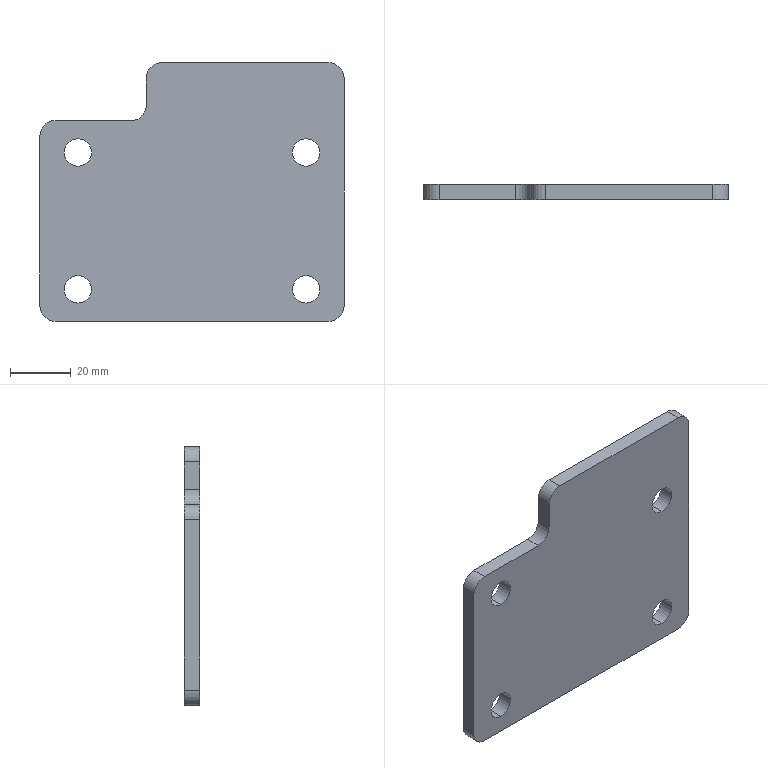Part | SolidWorks | features Fillet 2, Extrusion 1, HoleWzd 1, ICE 1 | 1 solid | 22 faces | box 100 x 5 x 85 mm | volume 37795 mm3 | cylinder 14 | plane 8 | commonest cylinder face diameters 9 x8 10 x6
STEP:
#1=CARTESIAN_POINT('',(-37.5,0.,-36.5));
#2=VERTEX_POINT('',#1);
#3=CARTESIAN_POINT('',(-37.5,0.,-27.5));
#4=VERTEX_POINT('',#3);
#5=CARTESIAN_POINT('',(-37.5,0.,-32.));
#6=DIRECTION('',(0.,1.,0.));
#7=DIRECTION('',(0.,0.,1.));
#8=AXIS2_PLACEMENT_3D('',#5,#6,#7);
#9=CIRCLE('',#8,4.5);
#10=EDGE_CURVE('',#2,#4,#9,.T.);
#11=ORIENTED_EDGE('',*,*,#10,.F.);
#12=CARTESIAN_POINT('',(-37.5,5.,-36.5));
#13=VERTEX_POINT('',#12);
#14=CARTESIAN_POINT('',(-37.5,5.,-36.5));
#15=DIRECTION('',(0.,1.,0.));
#16=VECTOR('',#15,1000.);
#17=LINE('',#14,#16);
#18=EDGE_CURVE('',#2,#13,#17,.T.);
#19=ORIENTED_EDGE('',*,*,#18,.T.);
#20=CARTESIAN_POINT('',(-37.5,5.,-27.5));
#21=VERTEX_POINT('',#20);
#22=CARTESIAN_POINT('',(-37.5,5.,-32.));
#23=DIRECTION('',(0.,1.,0.));
#24=DIRECTION('',(0.,0.,1.));
#25=AXIS2_PLACEMENT_3D('',#22,#23,#24);
#26=CIRCLE('',#25,4.5);
#27=EDGE_CURVE('',#13,#21,#26,.T.);
#28=ORIENTED_EDGE('',*,*,#27,.T.);
#29=CARTESIAN_POINT('',(-37.5,5.,-27.5));
#30=DIRECTION('',(0.,1.,0.));
#31=VECTOR('',#30,1000.);
#32=LINE('',#29,#31);
#33=EDGE_CURVE('',#4,#21,#32,.T.);
#34=ORIENTED_EDGE('',*,*,#33,.F.);
#35=EDGE_LOOP('',(#11,#19,#28,#34));
#36=FACE_OUTER_BOUND('',#35,.T.);
#37=CARTESIAN_POINT('',(-37.5,5.,-32.));
#38=DIRECTION('',(0.,1.,0.));
#39=DIRECTION('',(0.,0.,1.));
#40=AXIS2_PLACEMENT_3D('',#37,#38,#39);
#41=CYLINDRICAL_SURFACE('',#40,4.5);
#42=ADVANCED_FACE('',(#36),#41,.F.);
#43=CARTESIAN_POINT('',(37.5,0.,-36.5));
#44=VERTEX_POINT('',#43);
#45=CARTESIAN_POINT('',(37.5,0.,-27.5));
#46=VERTEX_POINT('',#45);
#47=CARTESIAN_POINT('',(37.5,0.,-32.));
#48=DIRECTION('',(0.,1.,0.));
#49=DIRECTION('',(0.,0.,1.));
#50=AXIS2_PLACEMENT_3D('',#47,#48,#49);
#51=CIRCLE('',#50,4.5);
#52=EDGE_CURVE('',#44,#46,#51,.T.);
#53=ORIENTED_EDGE('',*,*,#52,.F.);
#54=CARTESIAN_POINT('',(37.5,5.,-36.5));
#55=VERTEX_POINT('',#54);
#56=CARTESIAN_POINT('',(37.5,5.,-36.5));
#57=DIRECTION('',(0.,1.,0.));
#58=VECTOR('',#57,1000.);
#59=LINE('',#56,#58);
#60=EDGE_CURVE('',#44,#55,#59,.T.);
#61=ORIENTED_EDGE('',*,*,#60,.T.);
#62=CARTESIAN_POINT('',(37.5,5.,-27.5));
#63=VERTEX_POINT('',#62);
#64=CARTESIAN_POINT('',(37.5,5.,-32.));
#65=DIRECTION('',(0.,1.,0.));
#66=DIRECTION('',(0.,0.,1.));
#67=AXIS2_PLACEMENT_3D('',#64,#65,#66);
#68=CIRCLE('',#67,4.5);
#69=EDGE_CURVE('',#55,#63,#68,.T.);
#70=ORIENTED_EDGE('',*,*,#69,.T.);
#71=CARTESIAN_POINT('',(37.5,5.,-27.5));
#72=DIRECTION('',(0.,1.,0.));
#73=VECTOR('',#72,1000.);
#74=LINE('',#71,#73);
#75=EDGE_CURVE('',#46,#63,#74,.T.);
#76=ORIENTED_EDGE('',*,*,#75,.F.);
#77=EDGE_LOOP('',(#53,#61,#70,#76));
#78=FACE_OUTER_BOUND('',#77,.T.);
#79=CARTESIAN_POINT('',(37.5,5.,-32.));
#80=DIRECTION('',(0.,1.,0.));
#81=DIRECTION('',(0.,0.,1.));
#82=AXIS2_PLACEMENT_3D('',#79,#80,#81);
#83=CYLINDRICAL_SURFACE('',#82,4.5);
#84=ADVANCED_FACE('',(#78),#83,.F.);
#85=CARTESIAN_POINT('',(37.5,0.,8.5));
#86=VERTEX_POINT('',#85);
#87=CARTESIAN_POINT('',(37.5,0.,17.5));
#88=VERTEX_POINT('',#87);
#89=CARTESIAN_POINT('',(37.5,0.,13.));
#90=DIRECTION('',(0.,1.,0.));
#91=DIRECTION('',(0.,0.,1.));
#92=AXIS2_PLACEMENT_3D('',#89,#90,#91);
#93=CIRCLE('',#92,4.5);
#94=EDGE_CURVE('',#86,#88,#93,.T.);
#95=ORIENTED_EDGE('',*,*,#94,.F.);
#96=CARTESIAN_POINT('',(37.5,5.,8.5));
#97=VERTEX_POINT('',#96);
#98=CARTESIAN_POINT('',(37.5,5.,8.5));
#99=DIRECTION('',(0.,1.,0.));
#100=VECTOR('',#99,1000.);
#101=LINE('',#98,#100);
#102=EDGE_CURVE('',#86,#97,#101,.T.);
#103=ORIENTED_EDGE('',*,*,#102,.T.);
#104=CARTESIAN_POINT('',(37.5,5.,17.5));
#105=VERTEX_POINT('',#104);
#106=CARTESIAN_POINT('',(37.5,5.,13.));
#107=DIRECTION('',(0.,1.,0.));
#108=DIRECTION('',(0.,0.,1.));
#109=AXIS2_PLACEMENT_3D('',#106,#107,#108);
#110=CIRCLE('',#109,4.5);
#111=EDGE_CURVE('',#97,#105,#110,.T.);
#112=ORIENTED_EDGE('',*,*,#111,.T.);
#113=CARTESIAN_POINT('',(37.5,5.,17.5));
#114=DIRECTION('',(0.,1.,0.));
#115=VECTOR('',#114,1000.);
#116=LINE('',#113,#115);
#117=EDGE_CURVE('',#88,#105,#116,.T.);
#118=ORIENTED_EDGE('',*,*,#117,.F.);
#119=EDGE_LOOP('',(#95,#103,#112,#118));
#120=FACE_OUTER_BOUND('',#119,.T.);
#121=CARTESIAN_POINT('',(37.5,5.,13.));
#122=DIRECTION('',(0.,1.,0.));
#123=DIRECTION('',(0.,0.,1.));
#124=AXIS2_PLACEMENT_3D('',#121,#122,#123);
#125=CYLINDRICAL_SURFACE('',#124,4.5);
#126=ADVANCED_FACE('',(#120),#125,.F.);
#127=CARTESIAN_POINT('',(-37.5,0.,8.5));
#128=VERTEX_POINT('',#127);
#129=CARTESIAN_POINT('',(-37.5,0.,17.5));
#130=VERTEX_POINT('',#129);
#131=CARTESIAN_POINT('',(-37.5,0.,13.));
#132=DIRECTION('',(0.,1.,0.));
#133=DIRECTION('',(0.,0.,1.));
#134=AXIS2_PLACEMENT_3D('',#131,#132,#133);
#135=CIRCLE('',#134,4.5);
#136=EDGE_CURVE('',#128,#130,#135,.T.);
#137=ORIENTED_EDGE('',*,*,#136,.F.);
#138=CARTESIAN_POINT('',(-37.5,5.,8.5));
#139=VERTEX_POINT('',#138);
#140=CARTESIAN_POINT('',(-37.5,5.,8.5));
#141=DIRECTION('',(0.,1.,0.));
#142=VECTOR('',#141,1000.);
#143=LINE('',#140,#142);
#144=EDGE_CURVE('',#128,#139,#143,.T.);
#145=ORIENTED_EDGE('',*,*,#144,.T.);
#146=CARTESIAN_POINT('',(-37.5,5.,17.5));
#147=VERTEX_POINT('',#146);
#148=CARTESIAN_POINT('',(-37.5,5.,13.));
#149=DIRECTION('',(0.,1.,0.));
#150=DIRECTION('',(0.,0.,1.));
#151=AXIS2_PLACEMENT_3D('',#148,#149,#150);
#152=CIRCLE('',#151,4.5);
#153=EDGE_CURVE('',#139,#147,#152,.T.);
#154=ORIENTED_EDGE('',*,*,#153,.T.);
#155=CARTESIAN_POINT('',(-37.5,5.,17.5));
#156=DIRECTION('',(0.,1.,0.));
#157=VECTOR('',#156,1000.);
#158=LINE('',#155,#157);
#159=EDGE_CURVE('',#130,#147,#158,.T.);
#160=ORIENTED_EDGE('',*,*,#159,.F.);
#161=EDGE_LOOP('',(#137,#145,#154,#160));
#162=FACE_OUTER_BOUND('',#161,.T.);
#163=CARTESIAN_POINT('',(-37.5,5.,13.));
#164=DIRECTION('',(0.,1.,0.));
#165=DIRECTION('',(0.,0.,1.));
#166=AXIS2_PLACEMENT_3D('',#163,#164,#165);
#167=CYLINDRICAL_SURFACE('',#166,4.5);
#168=ADVANCED_FACE('',(#162),#167,.F.);
#169=CARTESIAN_POINT('',(50.,5.,37.5));
#170=VERTEX_POINT('',#169);
#171=CARTESIAN_POINT('',(50.,5.,-37.5));
#172=VERTEX_POINT('',#171);
#173=CARTESIAN_POINT('',(50.,5.,-42.5));
#174=DIRECTION('',(0.,0.,-1.));
#175=VECTOR('',#174,1000.);
#176=LINE('',#173,#175);
#177=EDGE_CURVE('',#170,#172,#176,.T.);
#178=ORIENTED_EDGE('',*,*,#177,.F.);
#179=CARTESIAN_POINT('',(50.,0.,37.5));
#180=VERTEX_POINT('',#179);
#181=CARTESIAN_POINT('',(50.,5.,37.5));
#182=DIRECTION('',(0.,-1.,0.));
#183=VECTOR('',#182,1000.);
#184=LINE('',#181,#183);
#185=EDGE_CURVE('',#170,#180,#184,.T.);
#186=ORIENTED_EDGE('',*,*,#185,.T.);
#187=CARTESIAN_POINT('',(50.,0.,-37.5));
#188=VERTEX_POINT('',#187);
#189=CARTESIAN_POINT('',(50.,0.,-42.5));
#190=DIRECTION('',(0.,0.,-1.));
#191=VECTOR('',#190,1000.);
#192=LINE('',#189,#191);
#193=EDGE_CURVE('',#180,#188,#192,.T.);
#194=ORIENTED_EDGE('',*,*,#193,.T.);
#195=CARTESIAN_POINT('',(50.,5.,-37.5));
#196=DIRECTION('',(0.,1.,0.));
#197=VECTOR('',#196,1000.);
#198=LINE('',#195,#197);
#199=EDGE_CURVE('',#188,#172,#198,.T.);
#200=ORIENTED_EDGE('',*,*,#199,.T.);
#201=EDGE_LOOP('',(#178,#186,#194,#200));
#202=FACE_OUTER_BOUND('',#201,.T.);
#203=CARTESIAN_POINT('',(50.,5.,-42.5));
#204=DIRECTION('',(-1.,0.,0.));
#205=DIRECTION('',(0.,0.,1.));
#206=AXIS2_PLACEMENT_3D('',#203,#204,#205);
#207=PLANE('',#206);
#208=ADVANCED_FACE('',(#202),#207,.F.);
#209=CARTESIAN_POINT('',(45.,5.,-42.5));
#210=VERTEX_POINT('',#209);
#211=CARTESIAN_POINT('',(-45.,5.,-42.5));
#212=VERTEX_POINT('',#211);
#213=CARTESIAN_POINT('',(-50.,5.,-42.5));
#214=DIRECTION('',(-1.,0.,0.));
#215=VECTOR('',#214,1000.);
#216=LINE('',#213,#215);
#217=EDGE_CURVE('',#210,#212,#216,.T.);
#218=ORIENTED_EDGE('',*,*,#217,.F.);
#219=CARTESIAN_POINT('',(45.,0.,-42.5));
#220=VERTEX_POINT('',#219);
#221=CARTESIAN_POINT('',(45.,5.,-42.5));
#222=DIRECTION('',(0.,-1.,0.));
#223=VECTOR('',#222,1000.);
#224=LINE('',#221,#223);
#225=EDGE_CURVE('',#210,#220,#224,.T.);
#226=ORIENTED_EDGE('',*,*,#225,.T.);
#227=CARTESIAN_POINT('',(-45.,0.,-42.5));
#228=VERTEX_POINT('',#227);
#229=CARTESIAN_POINT('',(-50.,0.,-42.5));
#230=DIRECTION('',(-1.,0.,0.));
#231=VECTOR('',#230,1000.);
#232=LINE('',#229,#231);
#233=EDGE_CURVE('',#220,#228,#232,.T.);
#234=ORIENTED_EDGE('',*,*,#233,.T.);
#235=CARTESIAN_POINT('',(-45.,5.,-42.5));
#236=DIRECTION('',(0.,1.,0.));
#237=VECTOR('',#236,1000.);
#238=LINE('',#235,#237);
#239=EDGE_CURVE('',#228,#212,#238,.T.);
#240=ORIENTED_EDGE('',*,*,#239,.T.);
#241=EDGE_LOOP('',(#218,#226,#234,#240));
#242=FACE_OUTER_BOUND('',#241,.T.);
#243=CARTESIAN_POINT('',(-50.,5.,-42.5));
#244=DIRECTION('',(0.,0.,1.));
#245=DIRECTION('',(1.,0.,0.));
#246=AXIS2_PLACEMENT_3D('',#243,#244,#245);
#247=PLANE('',#246);
#248=ADVANCED_FACE('',(#242),#247,.F.);
#249=CARTESIAN_POINT('',(-50.,0.,-37.5));
#250=VERTEX_POINT('',#249);
#251=CARTESIAN_POINT('',(-50.,0.,18.5));
#252=VERTEX_POINT('',#251);
#253=CARTESIAN_POINT('',(-50.,0.,-42.5));
#254=DIRECTION('',(0.,0.,1.));
#255=VECTOR('',#254,1000.);
#256=LINE('',#253,#255);
#257=EDGE_CURVE('',#250,#252,#256,.T.);
#258=ORIENTED_EDGE('',*,*,#257,.T.);
#259=CARTESIAN_POINT('',(-50.,5.,18.5));
#260=VERTEX_POINT('',#259);
#261=CARTESIAN_POINT('',(-50.,5.,18.5));
#262=DIRECTION('',(0.,1.,0.));
#263=VECTOR('',#262,1000.);
#264=LINE('',#261,#263);
#265=EDGE_CURVE('',#252,#260,#264,.T.);
#266=ORIENTED_EDGE('',*,*,#265,.T.);
#267=CARTESIAN_POINT('',(-50.,5.,-37.5));
#268=VERTEX_POINT('',#267);
#269=CARTESIAN_POINT('',(-50.,5.,-42.5));
#270=DIRECTION('',(0.,0.,1.));
#271=VECTOR('',#270,1000.);
#272=LINE('',#269,#271);
#273=EDGE_CURVE('',#268,#260,#272,.T.);
#274=ORIENTED_EDGE('',*,*,#273,.F.);
#275=CARTESIAN_POINT('',(-50.,5.,-37.5));
#276=DIRECTION('',(0.,-1.,0.));
#277=VECTOR('',#276,1000.);
#278=LINE('',#275,#277);
#279=EDGE_CURVE('',#268,#250,#278,.T.);
#280=ORIENTED_EDGE('',*,*,#279,.T.);
#281=EDGE_LOOP('',(#258,#266,#274,#280));
#282=FACE_OUTER_BOUND('',#281,.T.);
#283=CARTESIAN_POINT('',(-50.,5.,-42.5));
#284=DIRECTION('',(1.,0.,0.));
#285=DIRECTION('',(0.,0.,-1.));
#286=AXIS2_PLACEMENT_3D('',#283,#284,#285);
#287=PLANE('',#286);
#288=ADVANCED_FACE('',(#282),#287,.F.);
#289=CARTESIAN_POINT('',(-10.,5.,42.5));
#290=VERTEX_POINT('',#289);
#291=CARTESIAN_POINT('',(45.,5.,42.5));
#292=VERTEX_POINT('',#291);
#293=CARTESIAN_POINT('',(-50.,5.,42.5));
#294=DIRECTION('',(1.,0.,0.));
#295=VECTOR('',#294,1000.);
#296=LINE('',#293,#295);
#297=EDGE_CURVE('',#290,#292,#296,.T.);
#298=ORIENTED_EDGE('',*,*,#297,.F.);
#299=CARTESIAN_POINT('',(-10.,0.,42.5));
#300=VERTEX_POINT('',#299);
#301=CARTESIAN_POINT('',(-10.,5.,42.5));
#302=DIRECTION('',(0.,-1.,0.));
#303=VECTOR('',#302,1000.);
#304=LINE('',#301,#303);
#305=EDGE_CURVE('',#290,#300,#304,.T.);
#306=ORIENTED_EDGE('',*,*,#305,.T.);
#307=CARTESIAN_POINT('',(45.,0.,42.5));
#308=VERTEX_POINT('',#307);
#309=CARTESIAN_POINT('',(-50.,0.,42.5));
#310=DIRECTION('',(1.,0.,0.));
#311=VECTOR('',#310,1000.);
#312=LINE('',#309,#311);
#313=EDGE_CURVE('',#300,#308,#312,.T.);
#314=ORIENTED_EDGE('',*,*,#313,.T.);
#315=CARTESIAN_POINT('',(45.,5.,42.5));
#316=DIRECTION('',(0.,1.,0.));
#317=VECTOR('',#316,1000.);
#318=LINE('',#315,#317);
#319=EDGE_CURVE('',#308,#292,#318,.T.);
#320=ORIENTED_EDGE('',*,*,#319,.T.);
#321=EDGE_LOOP('',(#298,#306,#314,#320));
#322=FACE_OUTER_BOUND('',#321,.T.);
#323=CARTESIAN_POINT('',(-50.,5.,42.5));
#324=DIRECTION('',(0.,0.,-1.));
#325=DIRECTION('',(-1.,0.,0.));
#326=AXIS2_PLACEMENT_3D('',#323,#324,#325);
#327=PLANE('',#326);
#328=ADVANCED_FACE('',(#322),#327,.F.);
#329=CARTESIAN_POINT('',(-15.,5.,37.5));
#330=VERTEX_POINT('',#329);
#331=CARTESIAN_POINT('',(-15.,5.,28.5));
#332=VERTEX_POINT('',#331);
#333=CARTESIAN_POINT('',(-15.,5.,42.5));
#334=DIRECTION('',(0.,0.,-1.));
#335=VECTOR('',#334,1000.);
#336=LINE('',#333,#335);
#337=EDGE_CURVE('',#330,#332,#336,.T.);
#338=ORIENTED_EDGE('',*,*,#337,.F.);
#339=CARTESIAN_POINT('',(-10.,5.,37.5));
#340=DIRECTION('',(0.,1.,0.));
#341=DIRECTION('',(0.,0.,1.));
#342=AXIS2_PLACEMENT_3D('',#339,#340,#341);
#343=CIRCLE('',#342,5.);
#344=EDGE_CURVE('',#330,#290,#343,.T.);
#345=ORIENTED_EDGE('',*,*,#344,.T.);
#346=ORIENTED_EDGE('',*,*,#297,.T.);
#347=CARTESIAN_POINT('',(45.,5.,37.5));
#348=DIRECTION('',(0.,1.,0.));
#349=DIRECTION('',(0.,0.,1.));
#350=AXIS2_PLACEMENT_3D('',#347,#348,#349);
#351=CIRCLE('',#350,5.);
#352=EDGE_CURVE('',#292,#170,#351,.T.);
#353=ORIENTED_EDGE('',*,*,#352,.T.);
#354=ORIENTED_EDGE('',*,*,#177,.T.);
#355=CARTESIAN_POINT('',(45.,5.,-37.5));
#356=DIRECTION('',(0.,1.,0.));
#357=DIRECTION('',(0.,0.,1.));
#358=AXIS2_PLACEMENT_3D('',#355,#356,#357);
#359=CIRCLE('',#358,5.);
#360=EDGE_CURVE('',#172,#210,#359,.T.);
#361=ORIENTED_EDGE('',*,*,#360,.T.);
#362=ORIENTED_EDGE('',*,*,#217,.T.);
#363=CARTESIAN_POINT('',(-45.,5.,-37.5));
#364=DIRECTION('',(0.,1.,0.));
#365=DIRECTION('',(0.,0.,1.));
#366=AXIS2_PLACEMENT_3D('',#363,#364,#365);
#367=CIRCLE('',#366,5.);
#368=EDGE_CURVE('',#212,#268,#367,.T.);
#369=ORIENTED_EDGE('',*,*,#368,.T.);
#370=ORIENTED_EDGE('',*,*,#273,.T.);
#371=CARTESIAN_POINT('',(-45.,5.,23.5));
#372=VERTEX_POINT('',#371);
#373=CARTESIAN_POINT('',(-45.,5.,18.5));
#374=DIRECTION('',(0.,1.,0.));
#375=DIRECTION('',(0.,0.,1.));
#376=AXIS2_PLACEMENT_3D('',#373,#374,#375);
#377=CIRCLE('',#376,5.);
#378=EDGE_CURVE('',#260,#372,#377,.T.);
#379=ORIENTED_EDGE('',*,*,#378,.T.);
#380=CARTESIAN_POINT('',(-20.,5.,23.5));
#381=VERTEX_POINT('',#380);
#382=CARTESIAN_POINT('',(-50.,5.,23.5));
#383=DIRECTION('',(-1.,0.,0.));
#384=VECTOR('',#383,1000.);
#385=LINE('',#382,#384);
#386=EDGE_CURVE('',#381,#372,#385,.T.);
#387=ORIENTED_EDGE('',*,*,#386,.F.);
#388=CARTESIAN_POINT('',(-20.,5.,28.5));
#389=DIRECTION('',(0.,-1.,0.));
#390=DIRECTION('',(0.,0.,1.));
#391=AXIS2_PLACEMENT_3D('',#388,#389,#390);
#392=CIRCLE('',#391,5.);
#393=EDGE_CURVE('',#381,#332,#392,.T.);
#394=ORIENTED_EDGE('',*,*,#393,.T.);
#395=EDGE_LOOP('',(#338,#345,#346,#353,#354,#361,#362,#369,#370,#379,#387,#394));
#396=FACE_OUTER_BOUND('',#395,.T.);
#397=CARTESIAN_POINT('',(-37.5,5.,-32.));
#398=DIRECTION('',(0.,1.,0.));
#399=DIRECTION('',(0.,0.,1.));
#400=AXIS2_PLACEMENT_3D('',#397,#398,#399);
#401=CIRCLE('',#400,4.5);
#402=EDGE_CURVE('',#21,#13,#401,.T.);
#403=ORIENTED_EDGE('',*,*,#402,.F.);
#404=ORIENTED_EDGE('',*,*,#27,.F.);
#405=EDGE_LOOP('',(#403,#404));
#406=FACE_BOUND('',#405,.T.);
#407=CARTESIAN_POINT('',(37.5,5.,-32.));
#408=DIRECTION('',(0.,1.,0.));
#409=DIRECTION('',(0.,0.,1.));
#410=AXIS2_PLACEMENT_3D('',#407,#408,#409);
#411=CIRCLE('',#410,4.5);
#412=EDGE_CURVE('',#63,#55,#411,.T.);
#413=ORIENTED_EDGE('',*,*,#412,.F.);
#414=ORIENTED_EDGE('',*,*,#69,.F.);
#415=EDGE_LOOP('',(#413,#414));
#416=FACE_BOUND('',#415,.T.);
#417=CARTESIAN_POINT('',(37.5,5.,13.));
#418=DIRECTION('',(0.,1.,0.));
#419=DIRECTION('',(0.,0.,1.));
#420=AXIS2_PLACEMENT_3D('',#417,#418,#419);
#421=CIRCLE('',#420,4.5);
#422=EDGE_CURVE('',#105,#97,#421,.T.);
#423=ORIENTED_EDGE('',*,*,#422,.F.);
#424=ORIENTED_EDGE('',*,*,#111,.F.);
#425=EDGE_LOOP('',(#423,#424));
#426=FACE_BOUND('',#425,.T.);
#427=CARTESIAN_POINT('',(-37.5,5.,13.));
#428=DIRECTION('',(0.,1.,0.));
#429=DIRECTION('',(0.,0.,1.));
#430=AXIS2_PLACEMENT_3D('',#427,#428,#429);
#431=CIRCLE('',#430,4.5);
#432=EDGE_CURVE('',#147,#139,#431,.T.);
#433=ORIENTED_EDGE('',*,*,#432,.F.);
#434=ORIENTED_EDGE('',*,*,#153,.F.);
#435=EDGE_LOOP('',(#433,#434));
#436=FACE_BOUND('',#435,.T.);
#437=CARTESIAN_POINT('',(0.,5.,0.));
#438=DIRECTION('',(0.,1.,0.));
#439=DIRECTION('',(0.,0.,1.));
#440=AXIS2_PLACEMENT_3D('',#437,#438,#439);
#441=PLANE('',#440);
#442=ADVANCED_FACE('',(#396,#406,#416,#426,#436),#441,.T.);
#443=CARTESIAN_POINT('',(-37.5,0.,-32.));
#444=DIRECTION('',(0.,1.,0.));
#445=DIRECTION('',(0.,0.,1.));
#446=AXIS2_PLACEMENT_3D('',#443,#444,#445);
#447=CIRCLE('',#446,4.5);
#448=EDGE_CURVE('',#4,#2,#447,.T.);
#449=ORIENTED_EDGE('',*,*,#448,.T.);
#450=ORIENTED_EDGE('',*,*,#10,.T.);
#451=EDGE_LOOP('',(#449,#450));
#452=FACE_BOUND('',#451,.T.);
#453=CARTESIAN_POINT('',(37.5,0.,-32.));
#454=DIRECTION('',(0.,1.,0.));
#455=DIRECTION('',(0.,0.,1.));
#456=AXIS2_PLACEMENT_3D('',#453,#454,#455);
#457=CIRCLE('',#456,4.5);
#458=EDGE_CURVE('',#46,#44,#457,.T.);
#459=ORIENTED_EDGE('',*,*,#458,.T.);
#460=ORIENTED_EDGE('',*,*,#52,.T.);
#461=EDGE_LOOP('',(#459,#460));
#462=FACE_BOUND('',#461,.T.);
#463=CARTESIAN_POINT('',(37.5,0.,13.));
#464=DIRECTION('',(0.,1.,0.));
#465=DIRECTION('',(0.,0.,1.));
#466=AXIS2_PLACEMENT_3D('',#463,#464,#465);
#467=CIRCLE('',#466,4.5);
#468=EDGE_CURVE('',#88,#86,#467,.T.);
#469=ORIENTED_EDGE('',*,*,#468,.T.);
#470=ORIENTED_EDGE('',*,*,#94,.T.);
#471=EDGE_LOOP('',(#469,#470));
#472=FACE_BOUND('',#471,.T.);
#473=CARTESIAN_POINT('',(-37.5,0.,13.));
#474=DIRECTION('',(0.,1.,0.));
#475=DIRECTION('',(0.,0.,1.));
#476=AXIS2_PLACEMENT_3D('',#473,#474,#475);
#477=CIRCLE('',#476,4.5);
#478=EDGE_CURVE('',#130,#128,#477,.T.);
#479=ORIENTED_EDGE('',*,*,#478,.T.);
#480=ORIENTED_EDGE('',*,*,#136,.T.);
#481=EDGE_LOOP('',(#479,#480));
#482=FACE_BOUND('',#481,.T.);
#483=ORIENTED_EDGE('',*,*,#313,.F.);
#484=CARTESIAN_POINT('',(-15.,0.,37.5));
#485=VERTEX_POINT('',#484);
#486=CARTESIAN_POINT('',(-10.,0.,37.5));
#487=DIRECTION('',(0.,-1.,0.));
#488=DIRECTION('',(0.,0.,1.));
#489=AXIS2_PLACEMENT_3D('',#486,#487,#488);
#490=CIRCLE('',#489,5.);
#491=EDGE_CURVE('',#300,#485,#490,.T.);
#492=ORIENTED_EDGE('',*,*,#491,.T.);
#493=CARTESIAN_POINT('',(-15.,0.,28.5));
#494=VERTEX_POINT('',#493);
#495=CARTESIAN_POINT('',(-15.,0.,42.5));
#496=DIRECTION('',(0.,0.,-1.));
#497=VECTOR('',#496,1000.);
#498=LINE('',#495,#497);
#499=EDGE_CURVE('',#485,#494,#498,.T.);
#500=ORIENTED_EDGE('',*,*,#499,.T.);
#501=CARTESIAN_POINT('',(-20.,0.,23.5));
#502=VERTEX_POINT('',#501);
#503=CARTESIAN_POINT('',(-20.,0.,28.5));
#504=DIRECTION('',(0.,1.,0.));
#505=DIRECTION('',(0.,0.,1.));
#506=AXIS2_PLACEMENT_3D('',#503,#504,#505);
#507=CIRCLE('',#506,5.);
#508=EDGE_CURVE('',#494,#502,#507,.T.);
#509=ORIENTED_EDGE('',*,*,#508,.T.);
#510=CARTESIAN_POINT('',(-45.,0.,23.5));
#511=VERTEX_POINT('',#510);
#512=CARTESIAN_POINT('',(-50.,0.,23.5));
#513=DIRECTION('',(-1.,0.,0.));
#514=VECTOR('',#513,1000.);
#515=LINE('',#512,#514);
#516=EDGE_CURVE('',#502,#511,#515,.T.);
#517=ORIENTED_EDGE('',*,*,#516,.T.);
#518=CARTESIAN_POINT('',(-45.,0.,18.5));
#519=DIRECTION('',(0.,-1.,0.));
#520=DIRECTION('',(0.,0.,1.));
#521=AXIS2_PLACEMENT_3D('',#518,#519,#520);
#522=CIRCLE('',#521,5.);
#523=EDGE_CURVE('',#511,#252,#522,.T.);
#524=ORIENTED_EDGE('',*,*,#523,.T.);
#525=ORIENTED_EDGE('',*,*,#257,.F.);
#526=CARTESIAN_POINT('',(-45.,0.,-37.5));
#527=DIRECTION('',(0.,-1.,0.));
#528=DIRECTION('',(0.,0.,1.));
#529=AXIS2_PLACEMENT_3D('',#526,#527,#528);
#530=CIRCLE('',#529,5.);
#531=EDGE_CURVE('',#250,#228,#530,.T.);
#532=ORIENTED_EDGE('',*,*,#531,.T.);
#533=ORIENTED_EDGE('',*,*,#233,.F.);
#534=CARTESIAN_POINT('',(45.,0.,-37.5));
#535=DIRECTION('',(0.,-1.,0.));
#536=DIRECTION('',(0.,0.,1.));
#537=AXIS2_PLACEMENT_3D('',#534,#535,#536);
#538=CIRCLE('',#537,5.);
#539=EDGE_CURVE('',#220,#188,#538,.T.);
#540=ORIENTED_EDGE('',*,*,#539,.T.);
#541=ORIENTED_EDGE('',*,*,#193,.F.);
#542=CARTESIAN_POINT('',(45.,0.,37.5));
#543=DIRECTION('',(0.,-1.,0.));
#544=DIRECTION('',(0.,0.,1.));
#545=AXIS2_PLACEMENT_3D('',#542,#543,#544);
#546=CIRCLE('',#545,5.);
#547=EDGE_CURVE('',#180,#308,#546,.T.);
#548=ORIENTED_EDGE('',*,*,#547,.T.);
#549=EDGE_LOOP('',(#483,#492,#500,#509,#517,#524,#525,#532,#533,#540,#541,#548));
#550=FACE_OUTER_BOUND('',#549,.T.);
#551=CARTESIAN_POINT('',(0.,0.,0.));
#552=DIRECTION('',(0.,1.,0.));
#553=DIRECTION('',(0.,0.,1.));
#554=AXIS2_PLACEMENT_3D('',#551,#552,#553);
#555=PLANE('',#554);
#556=ADVANCED_FACE('',(#452,#462,#472,#482,#550),#555,.F.);
#557=ORIENTED_EDGE('',*,*,#144,.F.);
#558=ORIENTED_EDGE('',*,*,#478,.F.);
#559=ORIENTED_EDGE('',*,*,#159,.T.);
#560=ORIENTED_EDGE('',*,*,#432,.T.);
#561=EDGE_LOOP('',(#557,#558,#559,#560));
#562=FACE_OUTER_BOUND('',#561,.T.);
#563=CARTESIAN_POINT('',(-37.5,5.,13.));
#564=DIRECTION('',(0.,1.,0.));
#565=DIRECTION('',(0.,0.,1.));
#566=AXIS2_PLACEMENT_3D('',#563,#564,#565);
#567=CYLINDRICAL_SURFACE('',#566,4.5);
#568=ADVANCED_FACE('',(#562),#567,.F.);
#569=ORIENTED_EDGE('',*,*,#102,.F.);
#570=ORIENTED_EDGE('',*,*,#468,.F.);
#571=ORIENTED_EDGE('',*,*,#117,.T.);
#572=ORIENTED_EDGE('',*,*,#422,.T.);
#573=EDGE_LOOP('',(#569,#570,#571,#572));
#574=FACE_OUTER_BOUND('',#573,.T.);
#575=CARTESIAN_POINT('',(37.5,5.,13.));
#576=DIRECTION('',(0.,1.,0.));
#577=DIRECTION('',(0.,0.,1.));
#578=AXIS2_PLACEMENT_3D('',#575,#576,#577);
#579=CYLINDRICAL_SURFACE('',#578,4.5);
#580=ADVANCED_FACE('',(#574),#579,.F.);
#581=ORIENTED_EDGE('',*,*,#60,.F.);
#582=ORIENTED_EDGE('',*,*,#458,.F.);
#583=ORIENTED_EDGE('',*,*,#75,.T.);
#584=ORIENTED_EDGE('',*,*,#412,.T.);
#585=EDGE_LOOP('',(#581,#582,#583,#584));
#586=FACE_OUTER_BOUND('',#585,.T.);
#587=CARTESIAN_POINT('',(37.5,5.,-32.));
#588=DIRECTION('',(0.,1.,0.));
#589=DIRECTION('',(0.,0.,1.));
#590=AXIS2_PLACEMENT_3D('',#587,#588,#589);
#591=CYLINDRICAL_SURFACE('',#590,4.5);
#592=ADVANCED_FACE('',(#586),#591,.F.);
#593=ORIENTED_EDGE('',*,*,#18,.F.);
#594=ORIENTED_EDGE('',*,*,#448,.F.);
#595=ORIENTED_EDGE('',*,*,#33,.T.);
#596=ORIENTED_EDGE('',*,*,#402,.T.);
#597=EDGE_LOOP('',(#593,#594,#595,#596));
#598=FACE_OUTER_BOUND('',#597,.T.);
#599=CARTESIAN_POINT('',(-37.5,5.,-32.));
#600=DIRECTION('',(0.,1.,0.));
#601=DIRECTION('',(0.,0.,1.));
#602=AXIS2_PLACEMENT_3D('',#599,#600,#601);
#603=CYLINDRICAL_SURFACE('',#602,4.5);
#604=ADVANCED_FACE('',(#598),#603,.F.);
#605=ORIENTED_EDGE('',*,*,#352,.F.);
#606=ORIENTED_EDGE('',*,*,#319,.F.);
#607=ORIENTED_EDGE('',*,*,#547,.F.);
#608=ORIENTED_EDGE('',*,*,#185,.F.);
#609=EDGE_LOOP('',(#605,#606,#607,#608));
#610=FACE_OUTER_BOUND('',#609,.T.);
#611=CARTESIAN_POINT('',(45.,5.,37.5));
#612=DIRECTION('',(0.,-1.,0.));
#613=DIRECTION('',(0.,0.,-1.));
#614=AXIS2_PLACEMENT_3D('',#611,#612,#613);
#615=CYLINDRICAL_SURFACE('',#614,5.);
#616=ADVANCED_FACE('',(#610),#615,.T.);
#617=ORIENTED_EDGE('',*,*,#360,.F.);
#618=ORIENTED_EDGE('',*,*,#199,.F.);
#619=ORIENTED_EDGE('',*,*,#539,.F.);
#620=ORIENTED_EDGE('',*,*,#225,.F.);
#621=EDGE_LOOP('',(#617,#618,#619,#620));
#622=FACE_OUTER_BOUND('',#621,.T.);
#623=CARTESIAN_POINT('',(45.,5.,-37.5));
#624=DIRECTION('',(0.,-1.,0.));
#625=DIRECTION('',(0.,0.,-1.));
#626=AXIS2_PLACEMENT_3D('',#623,#624,#625);
#627=CYLINDRICAL_SURFACE('',#626,5.);
#628=ADVANCED_FACE('',(#622),#627,.T.);
#629=ORIENTED_EDGE('',*,*,#368,.F.);
#630=ORIENTED_EDGE('',*,*,#239,.F.);
#631=ORIENTED_EDGE('',*,*,#531,.F.);
#632=ORIENTED_EDGE('',*,*,#279,.F.);
#633=EDGE_LOOP('',(#629,#630,#631,#632));
#634=FACE_OUTER_BOUND('',#633,.T.);
#635=CARTESIAN_POINT('',(-45.,5.,-37.5));
#636=DIRECTION('',(0.,-1.,0.));
#637=DIRECTION('',(0.,0.,-1.));
#638=AXIS2_PLACEMENT_3D('',#635,#636,#637);
#639=CYLINDRICAL_SURFACE('',#638,5.);
#640=ADVANCED_FACE('',(#634),#639,.T.);
#641=ORIENTED_EDGE('',*,*,#516,.F.);
#642=CARTESIAN_POINT('',(-20.,5.,23.5));
#643=DIRECTION('',(0.,1.,0.));
#644=VECTOR('',#643,1000.);
#645=LINE('',#642,#644);
#646=EDGE_CURVE('',#502,#381,#645,.T.);
#647=ORIENTED_EDGE('',*,*,#646,.T.);
#648=ORIENTED_EDGE('',*,*,#386,.T.);
#649=CARTESIAN_POINT('',(-45.,0.,23.5));
#650=DIRECTION('',(0.,-1.,0.));
#651=VECTOR('',#650,1000.);
#652=LINE('',#649,#651);
#653=EDGE_CURVE('',#372,#511,#652,.T.);
#654=ORIENTED_EDGE('',*,*,#653,.T.);
#655=EDGE_LOOP('',(#641,#647,#648,#654));
#656=FACE_OUTER_BOUND('',#655,.T.);
#657=CARTESIAN_POINT('',(-50.,0.,23.5));
#658=DIRECTION('',(0.,0.,-1.));
#659=DIRECTION('',(-1.,0.,0.));
#660=AXIS2_PLACEMENT_3D('',#657,#658,#659);
#661=PLANE('',#660);
#662=ADVANCED_FACE('',(#656),#661,.F.);
#663=ORIENTED_EDGE('',*,*,#499,.F.);
#664=CARTESIAN_POINT('',(-15.,0.,37.5));
#665=DIRECTION('',(0.,1.,0.));
#666=VECTOR('',#665,1000.);
#667=LINE('',#664,#666);
#668=EDGE_CURVE('',#485,#330,#667,.T.);
#669=ORIENTED_EDGE('',*,*,#668,.T.);
#670=ORIENTED_EDGE('',*,*,#337,.T.);
#671=CARTESIAN_POINT('',(-15.,0.,28.5));
#672=DIRECTION('',(0.,-1.,0.));
#673=VECTOR('',#672,1000.);
#674=LINE('',#671,#673);
#675=EDGE_CURVE('',#332,#494,#674,.T.);
#676=ORIENTED_EDGE('',*,*,#675,.T.);
#677=EDGE_LOOP('',(#663,#669,#670,#676));
#678=FACE_OUTER_BOUND('',#677,.T.);
#679=CARTESIAN_POINT('',(-15.,0.,42.5));
#680=DIRECTION('',(1.,0.,0.));
#681=DIRECTION('',(0.,0.,-1.));
#682=AXIS2_PLACEMENT_3D('',#679,#680,#681);
#683=PLANE('',#682);
#684=ADVANCED_FACE('',(#678),#683,.F.);
#685=ORIENTED_EDGE('',*,*,#491,.F.);
#686=ORIENTED_EDGE('',*,*,#305,.F.);
#687=ORIENTED_EDGE('',*,*,#344,.F.);
#688=ORIENTED_EDGE('',*,*,#668,.F.);
#689=EDGE_LOOP('',(#685,#686,#687,#688));
#690=FACE_OUTER_BOUND('',#689,.T.);
#691=CARTESIAN_POINT('',(-10.,0.,37.5));
#692=DIRECTION('',(0.,1.,0.));
#693=DIRECTION('',(0.,0.,1.));
#694=AXIS2_PLACEMENT_3D('',#691,#692,#693);
#695=CYLINDRICAL_SURFACE('',#694,5.);
#696=ADVANCED_FACE('',(#690),#695,.T.);
#697=ORIENTED_EDGE('',*,*,#508,.F.);
#698=ORIENTED_EDGE('',*,*,#675,.F.);
#699=ORIENTED_EDGE('',*,*,#393,.F.);
#700=ORIENTED_EDGE('',*,*,#646,.F.);
#701=EDGE_LOOP('',(#697,#698,#699,#700));
#702=FACE_OUTER_BOUND('',#701,.T.);
#703=CARTESIAN_POINT('',(-20.,0.,28.5));
#704=DIRECTION('',(0.,-1.,0.));
#705=DIRECTION('',(0.,0.,-1.));
#706=AXIS2_PLACEMENT_3D('',#703,#704,#705);
#707=CYLINDRICAL_SURFACE('',#706,5.);
#708=ADVANCED_FACE('',(#702),#707,.F.);
#709=ORIENTED_EDGE('',*,*,#523,.F.);
#710=ORIENTED_EDGE('',*,*,#653,.F.);
#711=ORIENTED_EDGE('',*,*,#378,.F.);
#712=ORIENTED_EDGE('',*,*,#265,.F.);
#713=EDGE_LOOP('',(#709,#710,#711,#712));
#714=FACE_OUTER_BOUND('',#713,.T.);
#715=CARTESIAN_POINT('',(-45.,5.,18.5));
#716=DIRECTION('',(0.,1.,0.));
#717=DIRECTION('',(0.,0.,1.));
#718=AXIS2_PLACEMENT_3D('',#715,#716,#717);
#719=CYLINDRICAL_SURFACE('',#718,5.);
#720=ADVANCED_FACE('',(#714),#719,.T.);
#721=CLOSED_SHELL('',(#42,#84,#126,#168,#208,#248,#288,#328,#442,#556,#568,#580,#592,#604,#616,#628,#640,#662,#684,#696,#708,#720));
#722=MANIFOLD_SOLID_BREP('',#721);
#723=CARTESIAN_POINT('',(0.,0.,0.));
#724=DIRECTION('',(0.,0.,1.));
#725=DIRECTION('',(1.,0.,0.));
#726=AXIS2_PLACEMENT_3D('',#723,#724,#725);
#727=(LENGTH_UNIT()NAMED_UNIT(*)SI_UNIT(.MILLI.,.METRE.));
#728=UNCERTAINTY_MEASURE_WITH_UNIT(LENGTH_MEASURE(0.00001),#727,'','');
#729=(NAMED_UNIT(*)PLANE_ANGLE_UNIT()SI_UNIT($,.RADIAN.));
#730=(NAMED_UNIT(*)SI_UNIT($,.STERADIAN.)SOLID_ANGLE_UNIT());
#731=(GEOMETRIC_REPRESENTATION_CONTEXT(3)GLOBAL_UNCERTAINTY_ASSIGNED_CONTEXT((#728))GLOBAL_UNIT_ASSIGNED_CONTEXT((#727,#729,#730))REPRESENTATION_CONTEXT('',''));
#732=ADVANCED_BREP_SHAPE_REPRESENTATION('',(#722,#726),#731);